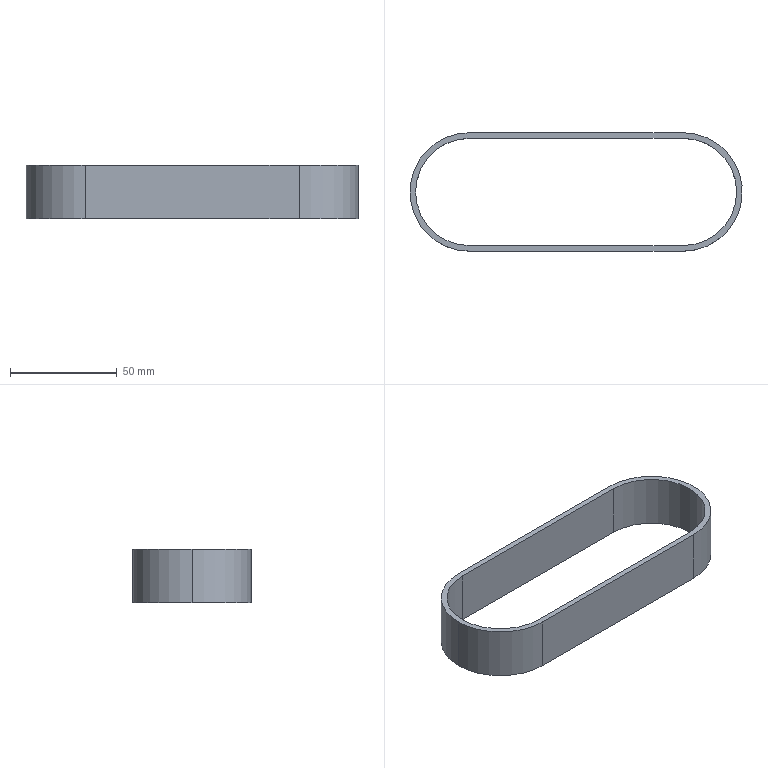Part | STEP file | Belt 1-5^ traction group | 1 solid | 12 faces | box 155.34 x 55.34 x 25 mm | volume 23948 mm3 | cylinder 6 | plane 6 | commonest cylinder face diameters 50.1 x3 55.34 x3
STEP:
#1=CARTESIAN_POINT('',(0.,0.,0.));
#2=DIRECTION('',(0.,0.,1.));
#3=DIRECTION('',(1.,0.,0.));
#4=AXIS2_PLACEMENT_3D('',#1,#2,#3);
#5=CARTESIAN_POINT('',(-82.918,-21.03,25.));
#6=VERTEX_POINT('',#5);
#7=CARTESIAN_POINT('',(-82.918,-21.03,0.));
#8=VERTEX_POINT('',#7);
#9=CARTESIAN_POINT('',(-82.918,-21.03,25.));
#10=DIRECTION('',(0.,0.,-1.));
#11=VECTOR('',#10,1.);
#12=LINE('',#9,#11);
#13=CARTESIAN_POINT('',(-82.918,-46.08,25.));
#14=DIRECTION('',(0.,0.,-1.));
#15=DIRECTION('',(-1.,0.,0.));
#16=AXIS2_PLACEMENT_3D('',#13,#14,#15);
#17=CYLINDRICAL_SURFACE('',#16,25.05);
#18=CARTESIAN_POINT('',(1.571,0.));
#19=DIRECTION('',(0.,1.));
#20=VECTOR('',#19,1.);
#21=LINE('',#18,#20);
#22=(GEOMETRIC_REPRESENTATION_CONTEXT(2)PARAMETRIC_REPRESENTATION_CONTEXT()REPRESENTATION_CONTEXT('',''));
#23=DEFINITIONAL_REPRESENTATION('',(#21),#22);
#24=PCURVE('',#17,#23);
#25=CARTESIAN_POINT('',(-82.918,-21.03,25.));
#26=DIRECTION('',(0.,1.,0.));
#27=DIRECTION('',(0.,0.,1.));
#28=AXIS2_PLACEMENT_3D('',#25,#26,#27);
#29=PLANE('',#28);
#30=CARTESIAN_POINT('',(0.,0.));
#31=DIRECTION('',(-1.,0.));
#32=VECTOR('',#31,1.);
#33=LINE('',#30,#32);
#34=(GEOMETRIC_REPRESENTATION_CONTEXT(2)PARAMETRIC_REPRESENTATION_CONTEXT()REPRESENTATION_CONTEXT('',''));
#35=DEFINITIONAL_REPRESENTATION('',(#33),#34);
#36=PCURVE('',#29,#35);
#37=SURFACE_CURVE('',#12,(#24,#36),.PCURVE_S1.);
#38=EDGE_CURVE('',#6,#8,#37,.T.);
#39=ORIENTED_EDGE('',*,*,#38,.T.);
#40=CARTESIAN_POINT('',(-107.968,-46.08,0.));
#41=VERTEX_POINT('',#40);
#42=CARTESIAN_POINT('',(-82.918,-46.08,0.));
#43=DIRECTION('',(0.,0.,-1.));
#44=DIRECTION('',(-1.,0.,0.));
#45=AXIS2_PLACEMENT_3D('',#42,#43,#44);
#46=CIRCLE('',#45,25.05);
#47=CARTESIAN_POINT('',(0.,25.));
#48=DIRECTION('',(1.,0.));
#49=VECTOR('',#48,1.);
#50=LINE('',#47,#49);
#51=(GEOMETRIC_REPRESENTATION_CONTEXT(2)PARAMETRIC_REPRESENTATION_CONTEXT()REPRESENTATION_CONTEXT('',''));
#52=DEFINITIONAL_REPRESENTATION('',(#50),#51);
#53=PCURVE('',#17,#52);
#54=CARTESIAN_POINT('',(-82.918,-46.08,0.));
#55=DIRECTION('',(0.,0.,-1.));
#56=DIRECTION('',(-1.,0.,0.));
#57=AXIS2_PLACEMENT_3D('',#54,#55,#56);
#58=PLANE('',#57);
#59=CARTESIAN_POINT('',(0.,0.));
#60=DIRECTION('',(1.,0.));
#61=AXIS2_PLACEMENT_2D('',#59,#60);
#62=CIRCLE('',#61,25.05);
#63=(GEOMETRIC_REPRESENTATION_CONTEXT(2)PARAMETRIC_REPRESENTATION_CONTEXT()REPRESENTATION_CONTEXT('',''));
#64=DEFINITIONAL_REPRESENTATION('',(#62),#63);
#65=PCURVE('',#58,#64);
#66=SURFACE_CURVE('',#46,(#53,#65),.PCURVE_S1.);
#67=EDGE_CURVE('',#41,#8,#66,.T.);
#68=ORIENTED_EDGE('',*,*,#67,.F.);
#69=CARTESIAN_POINT('',(-107.968,-46.08,25.));
#70=VERTEX_POINT('',#69);
#71=CARTESIAN_POINT('',(-107.968,-46.08,25.));
#72=DIRECTION('',(0.,0.,-1.));
#73=VECTOR('',#72,1.);
#74=LINE('',#71,#73);
#75=CARTESIAN_POINT('',(0.,0.));
#76=DIRECTION('',(0.,1.));
#77=VECTOR('',#76,1.);
#78=LINE('',#75,#77);
#79=(GEOMETRIC_REPRESENTATION_CONTEXT(2)PARAMETRIC_REPRESENTATION_CONTEXT()REPRESENTATION_CONTEXT('',''));
#80=DEFINITIONAL_REPRESENTATION('',(#78),#79);
#81=PCURVE('',#17,#80);
#82=CARTESIAN_POINT('',(-82.918,-46.08,25.));
#83=DIRECTION('',(0.,0.,-1.));
#84=DIRECTION('',(-1.,0.,0.));
#85=AXIS2_PLACEMENT_3D('',#82,#83,#84);
#86=CYLINDRICAL_SURFACE('',#85,25.05);
#87=CARTESIAN_POINT('',(6.283,0.));
#88=DIRECTION('',(0.,1.));
#89=VECTOR('',#88,1.);
#90=LINE('',#87,#89);
#91=(GEOMETRIC_REPRESENTATION_CONTEXT(2)PARAMETRIC_REPRESENTATION_CONTEXT()REPRESENTATION_CONTEXT('',''));
#92=DEFINITIONAL_REPRESENTATION('',(#90),#91);
#93=PCURVE('',#86,#92);
#94=SURFACE_CURVE('',#74,(#81,#93),.PCURVE_S1.);
#95=EDGE_CURVE('',#70,#41,#94,.T.);
#96=ORIENTED_EDGE('',*,*,#95,.F.);
#97=CARTESIAN_POINT('',(-82.918,-46.08,25.));
#98=DIRECTION('',(0.,0.,-1.));
#99=DIRECTION('',(-1.,0.,0.));
#100=AXIS2_PLACEMENT_3D('',#97,#98,#99);
#101=CIRCLE('',#100,25.05);
#102=CARTESIAN_POINT('',(0.,0.));
#103=DIRECTION('',(1.,0.));
#104=VECTOR('',#103,1.);
#105=LINE('',#102,#104);
#106=(GEOMETRIC_REPRESENTATION_CONTEXT(2)PARAMETRIC_REPRESENTATION_CONTEXT()REPRESENTATION_CONTEXT('',''));
#107=DEFINITIONAL_REPRESENTATION('',(#105),#106);
#108=PCURVE('',#17,#107);
#109=CARTESIAN_POINT('',(-82.918,-46.08,25.));
#110=DIRECTION('',(0.,0.,-1.));
#111=DIRECTION('',(-1.,0.,0.));
#112=AXIS2_PLACEMENT_3D('',#109,#110,#111);
#113=PLANE('',#112);
#114=CARTESIAN_POINT('',(0.,0.));
#115=DIRECTION('',(1.,0.));
#116=AXIS2_PLACEMENT_2D('',#114,#115);
#117=CIRCLE('',#116,25.05);
#118=(GEOMETRIC_REPRESENTATION_CONTEXT(2)PARAMETRIC_REPRESENTATION_CONTEXT()REPRESENTATION_CONTEXT('',''));
#119=DEFINITIONAL_REPRESENTATION('',(#117),#118);
#120=PCURVE('',#113,#119);
#121=SURFACE_CURVE('',#101,(#108,#120),.PCURVE_S1.);
#122=EDGE_CURVE('',#70,#6,#121,.T.);
#123=ORIENTED_EDGE('',*,*,#122,.T.);
#124=EDGE_LOOP('',(#39,#68,#96,#123));
#125=FACE_BOUND('',#124,.F.);
#126=ADVANCED_FACE('',(#125),#17,.F.);
#127=CARTESIAN_POINT('',(-82.918,-73.75,25.));
#128=VERTEX_POINT('',#127);
#129=CARTESIAN_POINT('',(-110.588,-46.08,25.));
#130=VERTEX_POINT('',#129);
#131=CARTESIAN_POINT('',(-82.918,-46.08,25.));
#132=DIRECTION('',(0.,0.,-1.));
#133=DIRECTION('',(-1.,0.,0.));
#134=AXIS2_PLACEMENT_3D('',#131,#132,#133);
#135=CIRCLE('',#134,27.67);
#136=CARTESIAN_POINT('',(-82.918,-46.08,25.));
#137=DIRECTION('',(0.,0.,-1.));
#138=DIRECTION('',(-1.,0.,0.));
#139=AXIS2_PLACEMENT_3D('',#136,#137,#138);
#140=CYLINDRICAL_SURFACE('',#139,27.67);
#141=CARTESIAN_POINT('',(0.,0.));
#142=DIRECTION('',(1.,0.));
#143=VECTOR('',#142,1.);
#144=LINE('',#141,#143);
#145=(GEOMETRIC_REPRESENTATION_CONTEXT(2)PARAMETRIC_REPRESENTATION_CONTEXT()REPRESENTATION_CONTEXT('',''));
#146=DEFINITIONAL_REPRESENTATION('',(#144),#145);
#147=PCURVE('',#140,#146);
#148=CARTESIAN_POINT('',(0.,0.));
#149=DIRECTION('',(1.,0.));
#150=AXIS2_PLACEMENT_2D('',#148,#149);
#151=CIRCLE('',#150,27.67);
#152=(GEOMETRIC_REPRESENTATION_CONTEXT(2)PARAMETRIC_REPRESENTATION_CONTEXT()REPRESENTATION_CONTEXT('',''));
#153=DEFINITIONAL_REPRESENTATION('',(#151),#152);
#154=PCURVE('',#113,#153);
#155=SURFACE_CURVE('',#135,(#147,#154),.PCURVE_S1.);
#156=EDGE_CURVE('',#128,#130,#155,.T.);
#157=ORIENTED_EDGE('',*,*,#156,.T.);
#158=CARTESIAN_POINT('',(-110.588,-46.08,0.));
#159=VERTEX_POINT('',#158);
#160=CARTESIAN_POINT('',(-110.588,-46.08,25.));
#161=DIRECTION('',(0.,0.,-1.));
#162=VECTOR('',#161,1.);
#163=LINE('',#160,#162);
#164=CARTESIAN_POINT('',(6.283,0.));
#165=DIRECTION('',(0.,1.));
#166=VECTOR('',#165,1.);
#167=LINE('',#164,#166);
#168=(GEOMETRIC_REPRESENTATION_CONTEXT(2)PARAMETRIC_REPRESENTATION_CONTEXT()REPRESENTATION_CONTEXT('',''));
#169=DEFINITIONAL_REPRESENTATION('',(#167),#168);
#170=PCURVE('',#140,#169);
#171=CARTESIAN_POINT('',(-82.918,-46.08,25.));
#172=DIRECTION('',(0.,0.,-1.));
#173=DIRECTION('',(-1.,0.,0.));
#174=AXIS2_PLACEMENT_3D('',#171,#172,#173);
#175=CYLINDRICAL_SURFACE('',#174,27.67);
#176=CARTESIAN_POINT('',(0.,0.));
#177=DIRECTION('',(0.,1.));
#178=VECTOR('',#177,1.);
#179=LINE('',#176,#178);
#180=(GEOMETRIC_REPRESENTATION_CONTEXT(2)PARAMETRIC_REPRESENTATION_CONTEXT()REPRESENTATION_CONTEXT('',''));
#181=DEFINITIONAL_REPRESENTATION('',(#179),#180);
#182=PCURVE('',#175,#181);
#183=SURFACE_CURVE('',#163,(#170,#182),.PCURVE_S1.);
#184=EDGE_CURVE('',#130,#159,#183,.T.);
#185=ORIENTED_EDGE('',*,*,#184,.T.);
#186=CARTESIAN_POINT('',(-82.918,-73.75,0.));
#187=VERTEX_POINT('',#186);
#188=CARTESIAN_POINT('',(-82.918,-46.08,0.));
#189=DIRECTION('',(0.,0.,-1.));
#190=DIRECTION('',(-1.,0.,0.));
#191=AXIS2_PLACEMENT_3D('',#188,#189,#190);
#192=CIRCLE('',#191,27.67);
#193=CARTESIAN_POINT('',(0.,25.));
#194=DIRECTION('',(1.,0.));
#195=VECTOR('',#194,1.);
#196=LINE('',#193,#195);
#197=(GEOMETRIC_REPRESENTATION_CONTEXT(2)PARAMETRIC_REPRESENTATION_CONTEXT()REPRESENTATION_CONTEXT('',''));
#198=DEFINITIONAL_REPRESENTATION('',(#196),#197);
#199=PCURVE('',#140,#198);
#200=CARTESIAN_POINT('',(0.,0.));
#201=DIRECTION('',(1.,0.));
#202=AXIS2_PLACEMENT_2D('',#200,#201);
#203=CIRCLE('',#202,27.67);
#204=(GEOMETRIC_REPRESENTATION_CONTEXT(2)PARAMETRIC_REPRESENTATION_CONTEXT()REPRESENTATION_CONTEXT('',''));
#205=DEFINITIONAL_REPRESENTATION('',(#203),#204);
#206=PCURVE('',#58,#205);
#207=SURFACE_CURVE('',#192,(#199,#206),.PCURVE_S1.);
#208=EDGE_CURVE('',#187,#159,#207,.T.);
#209=ORIENTED_EDGE('',*,*,#208,.F.);
#210=CARTESIAN_POINT('',(-82.918,-73.75,25.));
#211=DIRECTION('',(0.,0.,-1.));
#212=VECTOR('',#211,1.);
#213=LINE('',#210,#212);
#214=CARTESIAN_POINT('',(4.712,0.));
#215=DIRECTION('',(0.,1.));
#216=VECTOR('',#215,1.);
#217=LINE('',#214,#216);
#218=(GEOMETRIC_REPRESENTATION_CONTEXT(2)PARAMETRIC_REPRESENTATION_CONTEXT()REPRESENTATION_CONTEXT('',''));
#219=DEFINITIONAL_REPRESENTATION('',(#217),#218);
#220=PCURVE('',#140,#219);
#221=CARTESIAN_POINT('',(-82.918,-73.75,25.));
#222=DIRECTION('',(0.,-1.,0.));
#223=DIRECTION('',(0.,0.,-1.));
#224=AXIS2_PLACEMENT_3D('',#221,#222,#223);
#225=PLANE('',#224);
#226=CARTESIAN_POINT('',(0.,0.));
#227=DIRECTION('',(1.,0.));
#228=VECTOR('',#227,1.);
#229=LINE('',#226,#228);
#230=(GEOMETRIC_REPRESENTATION_CONTEXT(2)PARAMETRIC_REPRESENTATION_CONTEXT()REPRESENTATION_CONTEXT('',''));
#231=DEFINITIONAL_REPRESENTATION('',(#229),#230);
#232=PCURVE('',#225,#231);
#233=SURFACE_CURVE('',#213,(#220,#232),.PCURVE_S1.);
#234=EDGE_CURVE('',#128,#187,#233,.T.);
#235=ORIENTED_EDGE('',*,*,#234,.F.);
#236=EDGE_LOOP('',(#157,#185,#209,#235));
#237=FACE_BOUND('',#236,.T.);
#238=ADVANCED_FACE('',(#237),#140,.T.);
#239=ORIENTED_EDGE('',*,*,#184,.F.);
#240=CARTESIAN_POINT('',(-82.918,-18.41,25.));
#241=VERTEX_POINT('',#240);
#242=CARTESIAN_POINT('',(-82.918,-46.08,25.));
#243=DIRECTION('',(0.,0.,-1.));
#244=DIRECTION('',(-1.,0.,0.));
#245=AXIS2_PLACEMENT_3D('',#242,#243,#244);
#246=CIRCLE('',#245,27.67);
#247=CARTESIAN_POINT('',(0.,0.));
#248=DIRECTION('',(1.,0.));
#249=VECTOR('',#248,1.);
#250=LINE('',#247,#249);
#251=(GEOMETRIC_REPRESENTATION_CONTEXT(2)PARAMETRIC_REPRESENTATION_CONTEXT()REPRESENTATION_CONTEXT('',''));
#252=DEFINITIONAL_REPRESENTATION('',(#250),#251);
#253=PCURVE('',#175,#252);
#254=CARTESIAN_POINT('',(0.,0.));
#255=DIRECTION('',(1.,0.));
#256=AXIS2_PLACEMENT_2D('',#254,#255);
#257=CIRCLE('',#256,27.67);
#258=(GEOMETRIC_REPRESENTATION_CONTEXT(2)PARAMETRIC_REPRESENTATION_CONTEXT()REPRESENTATION_CONTEXT('',''));
#259=DEFINITIONAL_REPRESENTATION('',(#257),#258);
#260=PCURVE('',#113,#259);
#261=SURFACE_CURVE('',#246,(#253,#260),.PCURVE_S1.);
#262=EDGE_CURVE('',#130,#241,#261,.T.);
#263=ORIENTED_EDGE('',*,*,#262,.T.);
#264=CARTESIAN_POINT('',(-82.918,-18.41,0.));
#265=VERTEX_POINT('',#264);
#266=CARTESIAN_POINT('',(-82.918,-18.41,25.));
#267=DIRECTION('',(0.,0.,-1.));
#268=VECTOR('',#267,1.);
#269=LINE('',#266,#268);
#270=CARTESIAN_POINT('',(1.571,0.));
#271=DIRECTION('',(0.,1.));
#272=VECTOR('',#271,1.);
#273=LINE('',#270,#272);
#274=(GEOMETRIC_REPRESENTATION_CONTEXT(2)PARAMETRIC_REPRESENTATION_CONTEXT()REPRESENTATION_CONTEXT('',''));
#275=DEFINITIONAL_REPRESENTATION('',(#273),#274);
#276=PCURVE('',#175,#275);
#277=CARTESIAN_POINT('',(-82.918,-18.41,25.));
#278=DIRECTION('',(0.,1.,0.));
#279=DIRECTION('',(0.,0.,1.));
#280=AXIS2_PLACEMENT_3D('',#277,#278,#279);
#281=PLANE('',#280);
#282=CARTESIAN_POINT('',(0.,0.));
#283=DIRECTION('',(-1.,0.));
#284=VECTOR('',#283,1.);
#285=LINE('',#282,#284);
#286=(GEOMETRIC_REPRESENTATION_CONTEXT(2)PARAMETRIC_REPRESENTATION_CONTEXT()REPRESENTATION_CONTEXT('',''));
#287=DEFINITIONAL_REPRESENTATION('',(#285),#286);
#288=PCURVE('',#281,#287);
#289=SURFACE_CURVE('',#269,(#276,#288),.PCURVE_S1.);
#290=EDGE_CURVE('',#241,#265,#289,.T.);
#291=ORIENTED_EDGE('',*,*,#290,.T.);
#292=CARTESIAN_POINT('',(-82.918,-46.08,0.));
#293=DIRECTION('',(0.,0.,-1.));
#294=DIRECTION('',(-1.,0.,0.));
#295=AXIS2_PLACEMENT_3D('',#292,#293,#294);
#296=CIRCLE('',#295,27.67);
#297=CARTESIAN_POINT('',(0.,25.));
#298=DIRECTION('',(1.,0.));
#299=VECTOR('',#298,1.);
#300=LINE('',#297,#299);
#301=(GEOMETRIC_REPRESENTATION_CONTEXT(2)PARAMETRIC_REPRESENTATION_CONTEXT()REPRESENTATION_CONTEXT('',''));
#302=DEFINITIONAL_REPRESENTATION('',(#300),#301);
#303=PCURVE('',#175,#302);
#304=CARTESIAN_POINT('',(0.,0.));
#305=DIRECTION('',(1.,0.));
#306=AXIS2_PLACEMENT_2D('',#304,#305);
#307=CIRCLE('',#306,27.67);
#308=(GEOMETRIC_REPRESENTATION_CONTEXT(2)PARAMETRIC_REPRESENTATION_CONTEXT()REPRESENTATION_CONTEXT('',''));
#309=DEFINITIONAL_REPRESENTATION('',(#307),#308);
#310=PCURVE('',#58,#309);
#311=SURFACE_CURVE('',#296,(#303,#310),.PCURVE_S1.);
#312=EDGE_CURVE('',#159,#265,#311,.T.);
#313=ORIENTED_EDGE('',*,*,#312,.F.);
#314=EDGE_LOOP('',(#239,#263,#291,#313));
#315=FACE_BOUND('',#314,.T.);
#316=ADVANCED_FACE('',(#315),#175,.T.);
#317=CARTESIAN_POINT('',(17.082,-73.75,0.));
#318=VERTEX_POINT('',#317);
#319=CARTESIAN_POINT('',(-82.918,-73.75,0.));
#320=DIRECTION('',(-1.,0.,0.));
#321=VECTOR('',#320,1.);
#322=LINE('',#319,#321);
#323=CARTESIAN_POINT('',(25.,0.));
#324=DIRECTION('',(0.,-1.));
#325=VECTOR('',#324,1.);
#326=LINE('',#323,#325);
#327=(GEOMETRIC_REPRESENTATION_CONTEXT(2)PARAMETRIC_REPRESENTATION_CONTEXT()REPRESENTATION_CONTEXT('',''));
#328=DEFINITIONAL_REPRESENTATION('',(#326),#327);
#329=PCURVE('',#225,#328);
#330=CARTESIAN_POINT('',(0.,-27.67));
#331=DIRECTION('',(1.,0.));
#332=VECTOR('',#331,1.);
#333=LINE('',#330,#332);
#334=(GEOMETRIC_REPRESENTATION_CONTEXT(2)PARAMETRIC_REPRESENTATION_CONTEXT()REPRESENTATION_CONTEXT('',''));
#335=DEFINITIONAL_REPRESENTATION('',(#333),#334);
#336=PCURVE('',#58,#335);
#337=SURFACE_CURVE('',#322,(#329,#336),.PCURVE_S1.);
#338=EDGE_CURVE('',#318,#187,#337,.T.);
#339=ORIENTED_EDGE('',*,*,#338,.F.);
#340=CARTESIAN_POINT('',(17.082,-73.75,25.));
#341=VERTEX_POINT('',#340);
#342=CARTESIAN_POINT('',(17.082,-73.75,25.));
#343=DIRECTION('',(0.,0.,-1.));
#344=VECTOR('',#343,1.);
#345=LINE('',#342,#344);
#346=CARTESIAN_POINT('',(0.,100.));
#347=DIRECTION('',(1.,0.));
#348=VECTOR('',#347,1.);
#349=LINE('',#346,#348);
#350=(GEOMETRIC_REPRESENTATION_CONTEXT(2)PARAMETRIC_REPRESENTATION_CONTEXT()REPRESENTATION_CONTEXT('',''));
#351=DEFINITIONAL_REPRESENTATION('',(#349),#350);
#352=PCURVE('',#225,#351);
#353=CARTESIAN_POINT('',(17.082,-46.08,25.));
#354=DIRECTION('',(0.,0.,-1.));
#355=DIRECTION('',(-1.,0.,0.));
#356=AXIS2_PLACEMENT_3D('',#353,#354,#355);
#357=CYLINDRICAL_SURFACE('',#356,27.67);
#358=CARTESIAN_POINT('',(4.712,0.));
#359=DIRECTION('',(0.,1.));
#360=VECTOR('',#359,1.);
#361=LINE('',#358,#360);
#362=(GEOMETRIC_REPRESENTATION_CONTEXT(2)PARAMETRIC_REPRESENTATION_CONTEXT()REPRESENTATION_CONTEXT('',''));
#363=DEFINITIONAL_REPRESENTATION('',(#361),#362);
#364=PCURVE('',#357,#363);
#365=SURFACE_CURVE('',#345,(#352,#364),.PCURVE_S1.);
#366=EDGE_CURVE('',#341,#318,#365,.T.);
#367=ORIENTED_EDGE('',*,*,#366,.F.);
#368=CARTESIAN_POINT('',(-82.918,-73.75,25.));
#369=DIRECTION('',(-1.,0.,0.));
#370=VECTOR('',#369,1.);
#371=LINE('',#368,#370);
#372=CARTESIAN_POINT('',(0.,0.));
#373=DIRECTION('',(0.,-1.));
#374=VECTOR('',#373,1.);
#375=LINE('',#372,#374);
#376=(GEOMETRIC_REPRESENTATION_CONTEXT(2)PARAMETRIC_REPRESENTATION_CONTEXT()REPRESENTATION_CONTEXT('',''));
#377=DEFINITIONAL_REPRESENTATION('',(#375),#376);
#378=PCURVE('',#225,#377);
#379=CARTESIAN_POINT('',(0.,-27.67));
#380=DIRECTION('',(1.,0.));
#381=VECTOR('',#380,1.);
#382=LINE('',#379,#381);
#383=(GEOMETRIC_REPRESENTATION_CONTEXT(2)PARAMETRIC_REPRESENTATION_CONTEXT()REPRESENTATION_CONTEXT('',''));
#384=DEFINITIONAL_REPRESENTATION('',(#382),#383);
#385=PCURVE('',#113,#384);
#386=SURFACE_CURVE('',#371,(#378,#385),.PCURVE_S1.);
#387=EDGE_CURVE('',#341,#128,#386,.T.);
#388=ORIENTED_EDGE('',*,*,#387,.T.);
#389=ORIENTED_EDGE('',*,*,#234,.T.);
#390=EDGE_LOOP('',(#339,#367,#388,#389));
#391=FACE_BOUND('',#390,.T.);
#392=ADVANCED_FACE('',(#391),#225,.T.);
#393=CARTESIAN_POINT('',(17.082,-18.41,0.));
#394=VERTEX_POINT('',#393);
#395=CARTESIAN_POINT('',(17.082,-46.08,0.));
#396=DIRECTION('',(0.,0.,-1.));
#397=DIRECTION('',(-1.,0.,0.));
#398=AXIS2_PLACEMENT_3D('',#395,#396,#397);
#399=CIRCLE('',#398,27.67);
#400=CARTESIAN_POINT('',(0.,25.));
#401=DIRECTION('',(1.,0.));
#402=VECTOR('',#401,1.);
#403=LINE('',#400,#402);
#404=(GEOMETRIC_REPRESENTATION_CONTEXT(2)PARAMETRIC_REPRESENTATION_CONTEXT()REPRESENTATION_CONTEXT('',''));
#405=DEFINITIONAL_REPRESENTATION('',(#403),#404);
#406=PCURVE('',#357,#405);
#407=CARTESIAN_POINT('',(-100.,0.));
#408=DIRECTION('',(1.,0.));
#409=AXIS2_PLACEMENT_2D('',#407,#408);
#410=CIRCLE('',#409,27.67);
#411=(GEOMETRIC_REPRESENTATION_CONTEXT(2)PARAMETRIC_REPRESENTATION_CONTEXT()REPRESENTATION_CONTEXT('',''));
#412=DEFINITIONAL_REPRESENTATION('',(#410),#411);
#413=PCURVE('',#58,#412);
#414=SURFACE_CURVE('',#399,(#406,#413),.PCURVE_S1.);
#415=EDGE_CURVE('',#394,#318,#414,.T.);
#416=ORIENTED_EDGE('',*,*,#415,.F.);
#417=CARTESIAN_POINT('',(17.082,-18.41,25.));
#418=VERTEX_POINT('',#417);
#419=CARTESIAN_POINT('',(17.082,-18.41,25.));
#420=DIRECTION('',(0.,0.,-1.));
#421=VECTOR('',#420,1.);
#422=LINE('',#419,#421);
#423=CARTESIAN_POINT('',(1.571,0.));
#424=DIRECTION('',(0.,1.));
#425=VECTOR('',#424,1.);
#426=LINE('',#423,#425);
#427=(GEOMETRIC_REPRESENTATION_CONTEXT(2)PARAMETRIC_REPRESENTATION_CONTEXT()REPRESENTATION_CONTEXT('',''));
#428=DEFINITIONAL_REPRESENTATION('',(#426),#427);
#429=PCURVE('',#357,#428);
#430=CARTESIAN_POINT('',(0.,100.));
#431=DIRECTION('',(-1.,0.));
#432=VECTOR('',#431,1.);
#433=LINE('',#430,#432);
#434=(GEOMETRIC_REPRESENTATION_CONTEXT(2)PARAMETRIC_REPRESENTATION_CONTEXT()REPRESENTATION_CONTEXT('',''));
#435=DEFINITIONAL_REPRESENTATION('',(#433),#434);
#436=PCURVE('',#281,#435);
#437=SURFACE_CURVE('',#422,(#429,#436),.PCURVE_S1.);
#438=EDGE_CURVE('',#418,#394,#437,.T.);
#439=ORIENTED_EDGE('',*,*,#438,.F.);
#440=CARTESIAN_POINT('',(17.082,-46.08,25.));
#441=DIRECTION('',(0.,0.,-1.));
#442=DIRECTION('',(-1.,0.,0.));
#443=AXIS2_PLACEMENT_3D('',#440,#441,#442);
#444=CIRCLE('',#443,27.67);
#445=CARTESIAN_POINT('',(0.,0.));
#446=DIRECTION('',(1.,0.));
#447=VECTOR('',#446,1.);
#448=LINE('',#445,#447);
#449=(GEOMETRIC_REPRESENTATION_CONTEXT(2)PARAMETRIC_REPRESENTATION_CONTEXT()REPRESENTATION_CONTEXT('',''));
#450=DEFINITIONAL_REPRESENTATION('',(#448),#449);
#451=PCURVE('',#357,#450);
#452=CARTESIAN_POINT('',(-100.,0.));
#453=DIRECTION('',(1.,0.));
#454=AXIS2_PLACEMENT_2D('',#452,#453);
#455=CIRCLE('',#454,27.67);
#456=(GEOMETRIC_REPRESENTATION_CONTEXT(2)PARAMETRIC_REPRESENTATION_CONTEXT()REPRESENTATION_CONTEXT('',''));
#457=DEFINITIONAL_REPRESENTATION('',(#455),#456);
#458=PCURVE('',#113,#457);
#459=SURFACE_CURVE('',#444,(#451,#458),.PCURVE_S1.);
#460=EDGE_CURVE('',#418,#341,#459,.T.);
#461=ORIENTED_EDGE('',*,*,#460,.T.);
#462=ORIENTED_EDGE('',*,*,#366,.T.);
#463=EDGE_LOOP('',(#416,#439,#461,#462));
#464=FACE_BOUND('',#463,.T.);
#465=ADVANCED_FACE('',(#464),#357,.T.);
#466=CARTESIAN_POINT('',(-82.918,-18.41,0.));
#467=DIRECTION('',(1.,0.,0.));
#468=VECTOR('',#467,1.);
#469=LINE('',#466,#468);
#470=CARTESIAN_POINT('',(-25.,0.));
#471=DIRECTION('',(0.,1.));
#472=VECTOR('',#471,1.);
#473=LINE('',#470,#472);
#474=(GEOMETRIC_REPRESENTATION_CONTEXT(2)PARAMETRIC_REPRESENTATION_CONTEXT()REPRESENTATION_CONTEXT('',''));
#475=DEFINITIONAL_REPRESENTATION('',(#473),#474);
#476=PCURVE('',#281,#475);
#477=CARTESIAN_POINT('',(0.,27.67));
#478=DIRECTION('',(-1.,0.));
#479=VECTOR('',#478,1.);
#480=LINE('',#477,#479);
#481=(GEOMETRIC_REPRESENTATION_CONTEXT(2)PARAMETRIC_REPRESENTATION_CONTEXT()REPRESENTATION_CONTEXT('',''));
#482=DEFINITIONAL_REPRESENTATION('',(#480),#481);
#483=PCURVE('',#58,#482);
#484=SURFACE_CURVE('',#469,(#476,#483),.PCURVE_S1.);
#485=EDGE_CURVE('',#265,#394,#484,.T.);
#486=ORIENTED_EDGE('',*,*,#485,.F.);
#487=ORIENTED_EDGE('',*,*,#290,.F.);
#488=CARTESIAN_POINT('',(-82.918,-18.41,25.));
#489=DIRECTION('',(1.,0.,0.));
#490=VECTOR('',#489,1.);
#491=LINE('',#488,#490);
#492=CARTESIAN_POINT('',(0.,0.));
#493=DIRECTION('',(0.,1.));
#494=VECTOR('',#493,1.);
#495=LINE('',#492,#494);
#496=(GEOMETRIC_REPRESENTATION_CONTEXT(2)PARAMETRIC_REPRESENTATION_CONTEXT()REPRESENTATION_CONTEXT('',''));
#497=DEFINITIONAL_REPRESENTATION('',(#495),#496);
#498=PCURVE('',#281,#497);
#499=CARTESIAN_POINT('',(0.,27.67));
#500=DIRECTION('',(-1.,0.));
#501=VECTOR('',#500,1.);
#502=LINE('',#499,#501);
#503=(GEOMETRIC_REPRESENTATION_CONTEXT(2)PARAMETRIC_REPRESENTATION_CONTEXT()REPRESENTATION_CONTEXT('',''));
#504=DEFINITIONAL_REPRESENTATION('',(#502),#503);
#505=PCURVE('',#113,#504);
#506=SURFACE_CURVE('',#491,(#498,#505),.PCURVE_S1.);
#507=EDGE_CURVE('',#241,#418,#506,.T.);
#508=ORIENTED_EDGE('',*,*,#507,.T.);
#509=ORIENTED_EDGE('',*,*,#438,.T.);
#510=EDGE_LOOP('',(#486,#487,#508,#509));
#511=FACE_BOUND('',#510,.T.);
#512=ADVANCED_FACE('',(#511),#281,.T.);
#513=CARTESIAN_POINT('',(17.082,-71.13,25.));
#514=VERTEX_POINT('',#513);
#515=CARTESIAN_POINT('',(-82.918,-71.13,25.));
#516=VERTEX_POINT('',#515);
#517=CARTESIAN_POINT('',(17.082,-71.13,25.));
#518=DIRECTION('',(-1.,0.,0.));
#519=VECTOR('',#518,1.);
#520=LINE('',#517,#519);
#521=CARTESIAN_POINT('',(-100.,-25.05));
#522=DIRECTION('',(1.,0.));
#523=VECTOR('',#522,1.);
#524=LINE('',#521,#523);
#525=(GEOMETRIC_REPRESENTATION_CONTEXT(2)PARAMETRIC_REPRESENTATION_CONTEXT()REPRESENTATION_CONTEXT('',''));
#526=DEFINITIONAL_REPRESENTATION('',(#524),#525);
#527=PCURVE('',#113,#526);
#528=CARTESIAN_POINT('',(17.082,-71.13,25.));
#529=DIRECTION('',(0.,-1.,0.));
#530=DIRECTION('',(0.,0.,-1.));
#531=AXIS2_PLACEMENT_3D('',#528,#529,#530);
#532=PLANE('',#531);
#533=CARTESIAN_POINT('',(0.,0.));
#534=DIRECTION('',(0.,-1.));
#535=VECTOR('',#534,1.);
#536=LINE('',#533,#535);
#537=(GEOMETRIC_REPRESENTATION_CONTEXT(2)PARAMETRIC_REPRESENTATION_CONTEXT()REPRESENTATION_CONTEXT('',''));
#538=DEFINITIONAL_REPRESENTATION('',(#536),#537);
#539=PCURVE('',#532,#538);
#540=SURFACE_CURVE('',#520,(#527,#539),.PCURVE_S1.);
#541=EDGE_CURVE('',#514,#516,#540,.T.);
#542=ORIENTED_EDGE('',*,*,#541,.T.);
#543=CARTESIAN_POINT('',(-82.918,-46.08,25.));
#544=DIRECTION('',(0.,0.,-1.));
#545=DIRECTION('',(-1.,0.,0.));
#546=AXIS2_PLACEMENT_3D('',#543,#544,#545);
#547=CIRCLE('',#546,25.05);
#548=CARTESIAN_POINT('',(0.,0.));
#549=DIRECTION('',(1.,0.));
#550=AXIS2_PLACEMENT_2D('',#548,#549);
#551=CIRCLE('',#550,25.05);
#552=(GEOMETRIC_REPRESENTATION_CONTEXT(2)PARAMETRIC_REPRESENTATION_CONTEXT()REPRESENTATION_CONTEXT('',''));
#553=DEFINITIONAL_REPRESENTATION('',(#551),#552);
#554=PCURVE('',#113,#553);
#555=CARTESIAN_POINT('',(0.,0.));
#556=DIRECTION('',(1.,0.));
#557=VECTOR('',#556,1.);
#558=LINE('',#555,#557);
#559=(GEOMETRIC_REPRESENTATION_CONTEXT(2)PARAMETRIC_REPRESENTATION_CONTEXT()REPRESENTATION_CONTEXT('',''));
#560=DEFINITIONAL_REPRESENTATION('',(#558),#559);
#561=PCURVE('',#86,#560);
#562=SURFACE_CURVE('',#547,(#554,#561),.PCURVE_S1.);
#563=EDGE_CURVE('',#516,#70,#562,.T.);
#564=ORIENTED_EDGE('',*,*,#563,.T.);
#565=ORIENTED_EDGE('',*,*,#122,.T.);
#566=CARTESIAN_POINT('',(17.082,-21.03,25.));
#567=VERTEX_POINT('',#566);
#568=CARTESIAN_POINT('',(-82.918,-21.03,25.));
#569=DIRECTION('',(1.,0.,0.));
#570=VECTOR('',#569,1.);
#571=LINE('',#568,#570);
#572=CARTESIAN_POINT('',(0.,25.05));
#573=DIRECTION('',(-1.,0.));
#574=VECTOR('',#573,1.);
#575=LINE('',#572,#574);
#576=(GEOMETRIC_REPRESENTATION_CONTEXT(2)PARAMETRIC_REPRESENTATION_CONTEXT()REPRESENTATION_CONTEXT('',''));
#577=DEFINITIONAL_REPRESENTATION('',(#575),#576);
#578=PCURVE('',#113,#577);
#579=CARTESIAN_POINT('',(0.,0.));
#580=DIRECTION('',(0.,1.));
#581=VECTOR('',#580,1.);
#582=LINE('',#579,#581);
#583=(GEOMETRIC_REPRESENTATION_CONTEXT(2)PARAMETRIC_REPRESENTATION_CONTEXT()REPRESENTATION_CONTEXT('',''));
#584=DEFINITIONAL_REPRESENTATION('',(#582),#583);
#585=PCURVE('',#29,#584);
#586=SURFACE_CURVE('',#571,(#578,#585),.PCURVE_S1.);
#587=EDGE_CURVE('',#6,#567,#586,.T.);
#588=ORIENTED_EDGE('',*,*,#587,.T.);
#589=CARTESIAN_POINT('',(17.082,-46.08,25.));
#590=DIRECTION('',(0.,0.,-1.));
#591=DIRECTION('',(-1.,0.,0.));
#592=AXIS2_PLACEMENT_3D('',#589,#590,#591);
#593=CIRCLE('',#592,25.05);
#594=CARTESIAN_POINT('',(-100.,0.));
#595=DIRECTION('',(1.,0.));
#596=AXIS2_PLACEMENT_2D('',#594,#595);
#597=CIRCLE('',#596,25.05);
#598=(GEOMETRIC_REPRESENTATION_CONTEXT(2)PARAMETRIC_REPRESENTATION_CONTEXT()REPRESENTATION_CONTEXT('',''));
#599=DEFINITIONAL_REPRESENTATION('',(#597),#598);
#600=PCURVE('',#113,#599);
#601=CARTESIAN_POINT('',(17.082,-46.08,25.));
#602=DIRECTION('',(0.,0.,-1.));
#603=DIRECTION('',(-1.,0.,0.));
#604=AXIS2_PLACEMENT_3D('',#601,#602,#603);
#605=CYLINDRICAL_SURFACE('',#604,25.05);
#606=CARTESIAN_POINT('',(0.,0.));
#607=DIRECTION('',(1.,0.));
#608=VECTOR('',#607,1.);
#609=LINE('',#606,#608);
#610=(GEOMETRIC_REPRESENTATION_CONTEXT(2)PARAMETRIC_REPRESENTATION_CONTEXT()REPRESENTATION_CONTEXT('',''));
#611=DEFINITIONAL_REPRESENTATION('',(#609),#610);
#612=PCURVE('',#605,#611);
#613=SURFACE_CURVE('',#593,(#600,#612),.PCURVE_S1.);
#614=EDGE_CURVE('',#567,#514,#613,.T.);
#615=ORIENTED_EDGE('',*,*,#614,.T.);
#616=EDGE_LOOP('',(#542,#564,#565,#588,#615));
#617=FACE_BOUND('',#616,.T.);
#618=ORIENTED_EDGE('',*,*,#156,.F.);
#619=ORIENTED_EDGE('',*,*,#387,.F.);
#620=ORIENTED_EDGE('',*,*,#460,.F.);
#621=ORIENTED_EDGE('',*,*,#507,.F.);
#622=ORIENTED_EDGE('',*,*,#262,.F.);
#623=EDGE_LOOP('',(#618,#619,#620,#621,#622));
#624=FACE_BOUND('',#623,.T.);
#625=ADVANCED_FACE('',(#617,#624),#113,.F.);
#626=CARTESIAN_POINT('',(-82.918,-71.13,0.));
#627=VERTEX_POINT('',#626);
#628=CARTESIAN_POINT('',(-82.918,-46.08,0.));
#629=DIRECTION('',(0.,0.,-1.));
#630=DIRECTION('',(-1.,0.,0.));
#631=AXIS2_PLACEMENT_3D('',#628,#629,#630);
#632=CIRCLE('',#631,25.05);
#633=CARTESIAN_POINT('',(0.,0.));
#634=DIRECTION('',(1.,0.));
#635=AXIS2_PLACEMENT_2D('',#633,#634);
#636=CIRCLE('',#635,25.05);
#637=(GEOMETRIC_REPRESENTATION_CONTEXT(2)PARAMETRIC_REPRESENTATION_CONTEXT()REPRESENTATION_CONTEXT('',''));
#638=DEFINITIONAL_REPRESENTATION('',(#636),#637);
#639=PCURVE('',#58,#638);
#640=CARTESIAN_POINT('',(0.,25.));
#641=DIRECTION('',(1.,0.));
#642=VECTOR('',#641,1.);
#643=LINE('',#640,#642);
#644=(GEOMETRIC_REPRESENTATION_CONTEXT(2)PARAMETRIC_REPRESENTATION_CONTEXT()REPRESENTATION_CONTEXT('',''));
#645=DEFINITIONAL_REPRESENTATION('',(#643),#644);
#646=PCURVE('',#86,#645);
#647=SURFACE_CURVE('',#632,(#639,#646),.PCURVE_S1.);
#648=EDGE_CURVE('',#627,#41,#647,.T.);
#649=ORIENTED_EDGE('',*,*,#648,.F.);
#650=CARTESIAN_POINT('',(17.082,-71.13,0.));
#651=VERTEX_POINT('',#650);
#652=CARTESIAN_POINT('',(17.082,-71.13,0.));
#653=DIRECTION('',(-1.,0.,0.));
#654=VECTOR('',#653,1.);
#655=LINE('',#652,#654);
#656=CARTESIAN_POINT('',(-100.,-25.05));
#657=DIRECTION('',(1.,0.));
#658=VECTOR('',#657,1.);
#659=LINE('',#656,#658);
#660=(GEOMETRIC_REPRESENTATION_CONTEXT(2)PARAMETRIC_REPRESENTATION_CONTEXT()REPRESENTATION_CONTEXT('',''));
#661=DEFINITIONAL_REPRESENTATION('',(#659),#660);
#662=PCURVE('',#58,#661);
#663=CARTESIAN_POINT('',(25.,0.));
#664=DIRECTION('',(0.,-1.));
#665=VECTOR('',#664,1.);
#666=LINE('',#663,#665);
#667=(GEOMETRIC_REPRESENTATION_CONTEXT(2)PARAMETRIC_REPRESENTATION_CONTEXT()REPRESENTATION_CONTEXT('',''));
#668=DEFINITIONAL_REPRESENTATION('',(#666),#667);
#669=PCURVE('',#532,#668);
#670=SURFACE_CURVE('',#655,(#662,#669),.PCURVE_S1.);
#671=EDGE_CURVE('',#651,#627,#670,.T.);
#672=ORIENTED_EDGE('',*,*,#671,.F.);
#673=CARTESIAN_POINT('',(17.082,-21.03,0.));
#674=VERTEX_POINT('',#673);
#675=CARTESIAN_POINT('',(17.082,-46.08,0.));
#676=DIRECTION('',(0.,0.,-1.));
#677=DIRECTION('',(-1.,0.,0.));
#678=AXIS2_PLACEMENT_3D('',#675,#676,#677);
#679=CIRCLE('',#678,25.05);
#680=CARTESIAN_POINT('',(-100.,0.));
#681=DIRECTION('',(1.,0.));
#682=AXIS2_PLACEMENT_2D('',#680,#681);
#683=CIRCLE('',#682,25.05);
#684=(GEOMETRIC_REPRESENTATION_CONTEXT(2)PARAMETRIC_REPRESENTATION_CONTEXT()REPRESENTATION_CONTEXT('',''));
#685=DEFINITIONAL_REPRESENTATION('',(#683),#684);
#686=PCURVE('',#58,#685);
#687=CARTESIAN_POINT('',(0.,25.));
#688=DIRECTION('',(1.,0.));
#689=VECTOR('',#688,1.);
#690=LINE('',#687,#689);
#691=(GEOMETRIC_REPRESENTATION_CONTEXT(2)PARAMETRIC_REPRESENTATION_CONTEXT()REPRESENTATION_CONTEXT('',''));
#692=DEFINITIONAL_REPRESENTATION('',(#690),#691);
#693=PCURVE('',#605,#692);
#694=SURFACE_CURVE('',#679,(#686,#693),.PCURVE_S1.);
#695=EDGE_CURVE('',#674,#651,#694,.T.);
#696=ORIENTED_EDGE('',*,*,#695,.F.);
#697=CARTESIAN_POINT('',(-82.918,-21.03,0.));
#698=DIRECTION('',(1.,0.,0.));
#699=VECTOR('',#698,1.);
#700=LINE('',#697,#699);
#701=CARTESIAN_POINT('',(0.,25.05));
#702=DIRECTION('',(-1.,0.));
#703=VECTOR('',#702,1.);
#704=LINE('',#701,#703);
#705=(GEOMETRIC_REPRESENTATION_CONTEXT(2)PARAMETRIC_REPRESENTATION_CONTEXT()REPRESENTATION_CONTEXT('',''));
#706=DEFINITIONAL_REPRESENTATION('',(#704),#705);
#707=PCURVE('',#58,#706);
#708=CARTESIAN_POINT('',(-25.,0.));
#709=DIRECTION('',(0.,1.));
#710=VECTOR('',#709,1.);
#711=LINE('',#708,#710);
#712=(GEOMETRIC_REPRESENTATION_CONTEXT(2)PARAMETRIC_REPRESENTATION_CONTEXT()REPRESENTATION_CONTEXT('',''));
#713=DEFINITIONAL_REPRESENTATION('',(#711),#712);
#714=PCURVE('',#29,#713);
#715=SURFACE_CURVE('',#700,(#707,#714),.PCURVE_S1.);
#716=EDGE_CURVE('',#8,#674,#715,.T.);
#717=ORIENTED_EDGE('',*,*,#716,.F.);
#718=ORIENTED_EDGE('',*,*,#67,.F.);
#719=EDGE_LOOP('',(#649,#672,#696,#717,#718));
#720=FACE_BOUND('',#719,.T.);
#721=ORIENTED_EDGE('',*,*,#208,.T.);
#722=ORIENTED_EDGE('',*,*,#312,.T.);
#723=ORIENTED_EDGE('',*,*,#485,.T.);
#724=ORIENTED_EDGE('',*,*,#415,.T.);
#725=ORIENTED_EDGE('',*,*,#338,.T.);
#726=EDGE_LOOP('',(#721,#722,#723,#724,#725));
#727=FACE_BOUND('',#726,.T.);
#728=ADVANCED_FACE('',(#720,#727),#58,.T.);
#729=ORIENTED_EDGE('',*,*,#648,.F.);
#730=CARTESIAN_POINT('',(-82.918,-71.13,25.));
#731=DIRECTION('',(0.,0.,-1.));
#732=VECTOR('',#731,1.);
#733=LINE('',#730,#732);
#734=CARTESIAN_POINT('',(4.712,0.));
#735=DIRECTION('',(0.,1.));
#736=VECTOR('',#735,1.);
#737=LINE('',#734,#736);
#738=(GEOMETRIC_REPRESENTATION_CONTEXT(2)PARAMETRIC_REPRESENTATION_CONTEXT()REPRESENTATION_CONTEXT('',''));
#739=DEFINITIONAL_REPRESENTATION('',(#737),#738);
#740=PCURVE('',#86,#739);
#741=CARTESIAN_POINT('',(0.,-100.));
#742=DIRECTION('',(1.,0.));
#743=VECTOR('',#742,1.);
#744=LINE('',#741,#743);
#745=(GEOMETRIC_REPRESENTATION_CONTEXT(2)PARAMETRIC_REPRESENTATION_CONTEXT()REPRESENTATION_CONTEXT('',''));
#746=DEFINITIONAL_REPRESENTATION('',(#744),#745);
#747=PCURVE('',#532,#746);
#748=SURFACE_CURVE('',#733,(#740,#747),.PCURVE_S1.);
#749=EDGE_CURVE('',#516,#627,#748,.T.);
#750=ORIENTED_EDGE('',*,*,#749,.F.);
#751=ORIENTED_EDGE('',*,*,#563,.T.);
#752=ORIENTED_EDGE('',*,*,#95,.T.);
#753=EDGE_LOOP('',(#729,#750,#751,#752));
#754=FACE_BOUND('',#753,.F.);
#755=ADVANCED_FACE('',(#754),#86,.F.);
#756=ORIENTED_EDGE('',*,*,#671,.T.);
#757=ORIENTED_EDGE('',*,*,#749,.F.);
#758=ORIENTED_EDGE('',*,*,#541,.F.);
#759=CARTESIAN_POINT('',(17.082,-71.13,25.));
#760=DIRECTION('',(0.,0.,-1.));
#761=VECTOR('',#760,1.);
#762=LINE('',#759,#761);
#763=CARTESIAN_POINT('',(0.,0.));
#764=DIRECTION('',(1.,0.));
#765=VECTOR('',#764,1.);
#766=LINE('',#763,#765);
#767=(GEOMETRIC_REPRESENTATION_CONTEXT(2)PARAMETRIC_REPRESENTATION_CONTEXT()REPRESENTATION_CONTEXT('',''));
#768=DEFINITIONAL_REPRESENTATION('',(#766),#767);
#769=PCURVE('',#532,#768);
#770=CARTESIAN_POINT('',(4.712,0.));
#771=DIRECTION('',(0.,1.));
#772=VECTOR('',#771,1.);
#773=LINE('',#770,#772);
#774=(GEOMETRIC_REPRESENTATION_CONTEXT(2)PARAMETRIC_REPRESENTATION_CONTEXT()REPRESENTATION_CONTEXT('',''));
#775=DEFINITIONAL_REPRESENTATION('',(#773),#774);
#776=PCURVE('',#605,#775);
#777=SURFACE_CURVE('',#762,(#769,#776),.PCURVE_S1.);
#778=EDGE_CURVE('',#514,#651,#777,.T.);
#779=ORIENTED_EDGE('',*,*,#778,.T.);
#780=EDGE_LOOP('',(#756,#757,#758,#779));
#781=FACE_BOUND('',#780,.T.);
#782=ADVANCED_FACE('',(#781),#532,.F.);
#783=CARTESIAN_POINT('',(17.082,-21.03,25.));
#784=DIRECTION('',(0.,0.,-1.));
#785=VECTOR('',#784,1.);
#786=LINE('',#783,#785);
#787=CARTESIAN_POINT('',(1.571,0.));
#788=DIRECTION('',(0.,1.));
#789=VECTOR('',#788,1.);
#790=LINE('',#787,#789);
#791=(GEOMETRIC_REPRESENTATION_CONTEXT(2)PARAMETRIC_REPRESENTATION_CONTEXT()REPRESENTATION_CONTEXT('',''));
#792=DEFINITIONAL_REPRESENTATION('',(#790),#791);
#793=PCURVE('',#605,#792);
#794=CARTESIAN_POINT('',(0.,100.));
#795=DIRECTION('',(-1.,0.));
#796=VECTOR('',#795,1.);
#797=LINE('',#794,#796);
#798=(GEOMETRIC_REPRESENTATION_CONTEXT(2)PARAMETRIC_REPRESENTATION_CONTEXT()REPRESENTATION_CONTEXT('',''));
#799=DEFINITIONAL_REPRESENTATION('',(#797),#798);
#800=PCURVE('',#29,#799);
#801=SURFACE_CURVE('',#786,(#793,#800),.PCURVE_S1.);
#802=EDGE_CURVE('',#567,#674,#801,.T.);
#803=ORIENTED_EDGE('',*,*,#802,.F.);
#804=ORIENTED_EDGE('',*,*,#614,.T.);
#805=ORIENTED_EDGE('',*,*,#778,.T.);
#806=ORIENTED_EDGE('',*,*,#695,.F.);
#807=EDGE_LOOP('',(#803,#804,#805,#806));
#808=FACE_BOUND('',#807,.F.);
#809=ADVANCED_FACE('',(#808),#605,.F.);
#810=ORIENTED_EDGE('',*,*,#716,.T.);
#811=ORIENTED_EDGE('',*,*,#802,.F.);
#812=ORIENTED_EDGE('',*,*,#587,.F.);
#813=ORIENTED_EDGE('',*,*,#38,.T.);
#814=EDGE_LOOP('',(#810,#811,#812,#813));
#815=FACE_BOUND('',#814,.T.);
#816=ADVANCED_FACE('',(#815),#29,.F.);
#817=CLOSED_SHELL('',(#126,#238,#316,#392,#465,#512,#625,#728,#755,#782,#809,#816));
#818=MANIFOLD_SOLID_BREP('',#817);
#819=(LENGTH_UNIT()NAMED_UNIT(*)SI_UNIT(.MILLI.,.METRE.));
#820=UNCERTAINTY_MEASURE_WITH_UNIT(LENGTH_MEASURE(0.0000001),#819,'','');
#821=(NAMED_UNIT(*)PLANE_ANGLE_UNIT()SI_UNIT($,.RADIAN.));
#822=(NAMED_UNIT(*)SI_UNIT($,.STERADIAN.)SOLID_ANGLE_UNIT());
#823=(GEOMETRIC_REPRESENTATION_CONTEXT(3)GLOBAL_UNCERTAINTY_ASSIGNED_CONTEXT((#820))GLOBAL_UNIT_ASSIGNED_CONTEXT((#819,#821,#822))REPRESENTATION_CONTEXT('',''));
#824=ADVANCED_BREP_SHAPE_REPRESENTATION('',(#4,#818),#823);